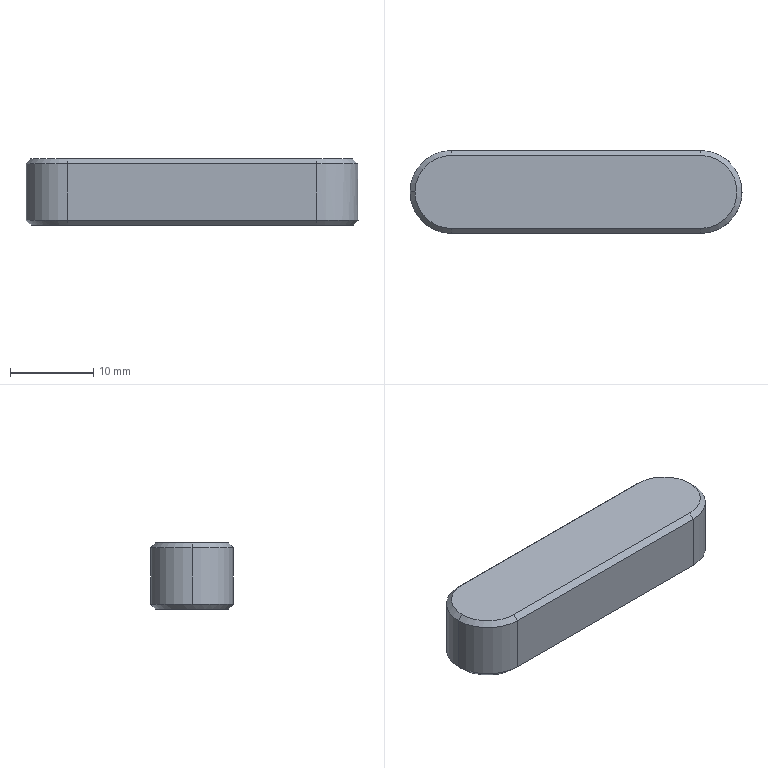Part | SolidWorks | features BaseBody 1 | 1 solid | 17 faces | box 40 x 10 x 8 mm | volume 2996 mm3 | plane 8 | cone 6 | cylinder 3 | commonest cylinder face diameters 10 x3
STEP:
#1=CARTESIAN_POINT('',(35.,-4.4,-5.));
#2=VERTEX_POINT('',#1);
#3=CARTESIAN_POINT('',(39.4,0.,-5.));
#4=VERTEX_POINT('',#3);
#5=CARTESIAN_POINT('',(35.,0.,-5.));
#6=DIRECTION('',(0.,0.,1.));
#7=DIRECTION('',(1.,0.,0.));
#8=AXIS2_PLACEMENT_3D('',#5,#6,#7);
#9=CIRCLE('',#8,4.4);
#10=EDGE_CURVE('',#2,#4,#9,.T.);
#11=ORIENTED_EDGE('',*,*,#10,.T.);
#12=CARTESIAN_POINT('',(40.,0.,-4.4));
#13=VERTEX_POINT('',#12);
#14=CARTESIAN_POINT('',(40.,0.,-4.4));
#15=DIRECTION('',(0.7071,0.,0.7071));
#16=VECTOR('',#15,1000.);
#17=LINE('',#14,#16);
#18=EDGE_CURVE('',#4,#13,#17,.T.);
#19=ORIENTED_EDGE('',*,*,#18,.T.);
#20=CARTESIAN_POINT('',(35.,-5.,-4.4));
#21=VERTEX_POINT('',#20);
#22=CARTESIAN_POINT('',(35.,0.,-4.4));
#23=DIRECTION('',(0.,0.,-1.));
#24=DIRECTION('',(0.,1.,0.));
#25=AXIS2_PLACEMENT_3D('',#22,#23,#24);
#26=CIRCLE('',#25,5.);
#27=EDGE_CURVE('',#13,#21,#26,.T.);
#28=ORIENTED_EDGE('',*,*,#27,.T.);
#29=CARTESIAN_POINT('',(35.,-4.7,-4.7));
#30=DIRECTION('',(0.,-0.7071,0.7071));
#31=VECTOR('',#30,1000.);
#32=LINE('',#29,#31);
#33=EDGE_CURVE('',#2,#21,#32,.T.);
#34=ORIENTED_EDGE('',*,*,#33,.F.);
#35=EDGE_LOOP('',(#11,#19,#28,#34));
#36=FACE_OUTER_BOUND('',#35,.T.);
#37=CARTESIAN_POINT('',(35.,0.,-4.4));
#38=DIRECTION('',(0.,0.,1.));
#39=DIRECTION('',(1.,0.,0.));
#40=AXIS2_PLACEMENT_3D('',#37,#38,#39);
#41=CONICAL_SURFACE('',#40,5.,0.7854);
#42=ADVANCED_FACE('',(#36),#41,.T.);
#43=CARTESIAN_POINT('',(5.,-5.,2.4));
#44=VERTEX_POINT('',#43);
#45=CARTESIAN_POINT('',(0.,0.,2.4));
#46=VERTEX_POINT('',#45);
#47=CARTESIAN_POINT('',(5.,0.,2.4));
#48=DIRECTION('',(0.,0.,-1.));
#49=DIRECTION('',(-1.,0.,0.));
#50=AXIS2_PLACEMENT_3D('',#47,#48,#49);
#51=CIRCLE('',#50,5.);
#52=EDGE_CURVE('',#44,#46,#51,.T.);
#53=ORIENTED_EDGE('',*,*,#52,.T.);
#54=CARTESIAN_POINT('',(0.,0.,-4.4));
#55=VERTEX_POINT('',#54);
#56=CARTESIAN_POINT('',(0.,0.,0.));
#57=DIRECTION('',(0.,0.,-1.));
#58=VECTOR('',#57,1000.);
#59=LINE('',#56,#58);
#60=EDGE_CURVE('',#46,#55,#59,.T.);
#61=ORIENTED_EDGE('',*,*,#60,.T.);
#62=CARTESIAN_POINT('',(5.,-5.,-4.4));
#63=VERTEX_POINT('',#62);
#64=CARTESIAN_POINT('',(5.,0.,-4.4));
#65=DIRECTION('',(0.,0.,-1.));
#66=DIRECTION('',(0.,-1.,0.));
#67=AXIS2_PLACEMENT_3D('',#64,#65,#66);
#68=CIRCLE('',#67,5.);
#69=EDGE_CURVE('',#63,#55,#68,.T.);
#70=ORIENTED_EDGE('',*,*,#69,.F.);
#71=CARTESIAN_POINT('',(5.,-5.,0.));
#72=DIRECTION('',(0.,0.,-1.));
#73=VECTOR('',#72,1000.);
#74=LINE('',#71,#73);
#75=EDGE_CURVE('',#44,#63,#74,.T.);
#76=ORIENTED_EDGE('',*,*,#75,.F.);
#77=EDGE_LOOP('',(#53,#61,#70,#76));
#78=FACE_OUTER_BOUND('',#77,.T.);
#79=CARTESIAN_POINT('',(5.,0.,0.));
#80=DIRECTION('',(0.,0.,-1.));
#81=DIRECTION('',(-1.,0.,0.));
#82=AXIS2_PLACEMENT_3D('',#79,#80,#81);
#83=CYLINDRICAL_SURFACE('',#82,5.);
#84=ADVANCED_FACE('',(#78),#83,.T.);
#85=CARTESIAN_POINT('',(5.,-4.4,3.));
#86=VERTEX_POINT('',#85);
#87=CARTESIAN_POINT('',(0.6,0.,3.));
#88=VERTEX_POINT('',#87);
#89=CARTESIAN_POINT('',(5.,0.,3.));
#90=DIRECTION('',(0.,0.,-1.));
#91=DIRECTION('',(-1.,0.,0.));
#92=AXIS2_PLACEMENT_3D('',#89,#90,#91);
#93=CIRCLE('',#92,4.4);
#94=EDGE_CURVE('',#86,#88,#93,.T.);
#95=ORIENTED_EDGE('',*,*,#94,.T.);
#96=CARTESIAN_POINT('',(0.,0.,2.4));
#97=DIRECTION('',(-0.7071,0.,-0.7071));
#98=VECTOR('',#97,1000.);
#99=LINE('',#96,#98);
#100=EDGE_CURVE('',#88,#46,#99,.T.);
#101=ORIENTED_EDGE('',*,*,#100,.T.);
#102=ORIENTED_EDGE('',*,*,#52,.F.);
#103=CARTESIAN_POINT('',(5.,-4.7,2.7));
#104=DIRECTION('',(0.,-0.7071,-0.7071));
#105=VECTOR('',#104,1000.);
#106=LINE('',#103,#105);
#107=EDGE_CURVE('',#86,#44,#106,.T.);
#108=ORIENTED_EDGE('',*,*,#107,.F.);
#109=EDGE_LOOP('',(#95,#101,#102,#108));
#110=FACE_OUTER_BOUND('',#109,.T.);
#111=CARTESIAN_POINT('',(5.,0.,2.4));
#112=DIRECTION('',(0.,0.,-1.));
#113=DIRECTION('',(-1.,0.,0.));
#114=AXIS2_PLACEMENT_3D('',#111,#112,#113);
#115=CONICAL_SURFACE('',#114,5.,0.7854);
#116=ADVANCED_FACE('',(#110),#115,.T.);
#117=CARTESIAN_POINT('',(5.,4.4,-5.));
#118=VERTEX_POINT('',#117);
#119=CARTESIAN_POINT('',(5.,-4.4,-5.));
#120=VERTEX_POINT('',#119);
#121=CARTESIAN_POINT('',(5.,0.,-5.));
#122=DIRECTION('',(0.,0.,1.));
#123=DIRECTION('',(1.,0.,0.));
#124=AXIS2_PLACEMENT_3D('',#121,#122,#123);
#125=CIRCLE('',#124,4.4);
#126=EDGE_CURVE('',#118,#120,#125,.T.);
#127=ORIENTED_EDGE('',*,*,#126,.F.);
#128=CARTESIAN_POINT('',(35.,4.4,-5.));
#129=VERTEX_POINT('',#128);
#130=CARTESIAN_POINT('',(20.,4.4,-5.));
#131=DIRECTION('',(-1.,0.,0.));
#132=VECTOR('',#131,1000.);
#133=LINE('',#130,#132);
#134=EDGE_CURVE('',#129,#118,#133,.T.);
#135=ORIENTED_EDGE('',*,*,#134,.F.);
#136=CARTESIAN_POINT('',(35.,0.,-5.));
#137=DIRECTION('',(0.,0.,1.));
#138=DIRECTION('',(1.,0.,0.));
#139=AXIS2_PLACEMENT_3D('',#136,#137,#138);
#140=CIRCLE('',#139,4.4);
#141=EDGE_CURVE('',#4,#129,#140,.T.);
#142=ORIENTED_EDGE('',*,*,#141,.F.);
#143=ORIENTED_EDGE('',*,*,#10,.F.);
#144=CARTESIAN_POINT('',(20.,-4.4,-5.));
#145=DIRECTION('',(1.,0.,0.));
#146=VECTOR('',#145,1000.);
#147=LINE('',#144,#146);
#148=EDGE_CURVE('',#120,#2,#147,.T.);
#149=ORIENTED_EDGE('',*,*,#148,.F.);
#150=EDGE_LOOP('',(#127,#135,#142,#143,#149));
#151=FACE_OUTER_BOUND('',#150,.T.);
#152=CARTESIAN_POINT('',(20.,0.,-5.));
#153=DIRECTION('',(0.,0.,1.));
#154=DIRECTION('',(1.,0.,0.));
#155=AXIS2_PLACEMENT_3D('',#152,#153,#154);
#156=PLANE('',#155);
#157=ADVANCED_FACE('',(#151),#156,.F.);
#158=CARTESIAN_POINT('',(5.,-4.7,-4.7));
#159=DIRECTION('',(0.,0.7071,-0.7071));
#160=VECTOR('',#159,1000.);
#161=LINE('',#158,#160);
#162=EDGE_CURVE('',#63,#120,#161,.T.);
#163=ORIENTED_EDGE('',*,*,#162,.T.);
#164=ORIENTED_EDGE('',*,*,#148,.T.);
#165=ORIENTED_EDGE('',*,*,#33,.T.);
#166=CARTESIAN_POINT('',(12.5,-5.,-4.4));
#167=DIRECTION('',(-1.,0.,0.));
#168=VECTOR('',#167,1000.);
#169=LINE('',#166,#168);
#170=EDGE_CURVE('',#21,#63,#169,.T.);
#171=ORIENTED_EDGE('',*,*,#170,.T.);
#172=EDGE_LOOP('',(#163,#164,#165,#171));
#173=FACE_OUTER_BOUND('',#172,.T.);
#174=CARTESIAN_POINT('',(12.5,-4.7,-4.7));
#175=DIRECTION('',(0.,-0.7071,-0.7071));
#176=DIRECTION('',(0.,0.7071,-0.7071));
#177=AXIS2_PLACEMENT_3D('',#174,#175,#176);
#178=PLANE('',#177);
#179=ADVANCED_FACE('',(#173),#178,.T.);
#180=ORIENTED_EDGE('',*,*,#162,.F.);
#181=ORIENTED_EDGE('',*,*,#69,.T.);
#182=CARTESIAN_POINT('',(5.,5.,-4.4));
#183=VERTEX_POINT('',#182);
#184=CARTESIAN_POINT('',(5.,0.,-4.4));
#185=DIRECTION('',(0.,0.,-1.));
#186=DIRECTION('',(0.,-1.,0.));
#187=AXIS2_PLACEMENT_3D('',#184,#185,#186);
#188=CIRCLE('',#187,5.);
#189=EDGE_CURVE('',#55,#183,#188,.T.);
#190=ORIENTED_EDGE('',*,*,#189,.T.);
#191=CARTESIAN_POINT('',(5.,499000.,498990.6));
#192=DIRECTION('',(0.,-0.7071,-0.7071));
#193=VECTOR('',#192,1000.);
#194=LINE('',#191,#193);
#195=EDGE_CURVE('',#183,#118,#194,.T.);
#196=ORIENTED_EDGE('',*,*,#195,.T.);
#197=ORIENTED_EDGE('',*,*,#126,.T.);
#198=EDGE_LOOP('',(#180,#181,#190,#196,#197));
#199=FACE_OUTER_BOUND('',#198,.T.);
#200=CARTESIAN_POINT('',(5.,0.,-4.4));
#201=DIRECTION('',(0.,0.,1.));
#202=DIRECTION('',(1.,0.,0.));
#203=AXIS2_PLACEMENT_3D('',#200,#201,#202);
#204=CONICAL_SURFACE('',#203,5.,0.7854);
#205=ADVANCED_FACE('',(#199),#204,.T.);
#206=ORIENTED_EDGE('',*,*,#195,.F.);
#207=CARTESIAN_POINT('',(35.,5.,-4.4));
#208=VERTEX_POINT('',#207);
#209=CARTESIAN_POINT('',(27.5,5.,-4.4));
#210=DIRECTION('',(1.,0.,0.));
#211=VECTOR('',#210,1000.);
#212=LINE('',#209,#211);
#213=EDGE_CURVE('',#183,#208,#212,.T.);
#214=ORIENTED_EDGE('',*,*,#213,.T.);
#215=CARTESIAN_POINT('',(35.,4.7,-4.7));
#216=DIRECTION('',(0.,-0.7071,-0.7071));
#217=VECTOR('',#216,1000.);
#218=LINE('',#215,#217);
#219=EDGE_CURVE('',#208,#129,#218,.T.);
#220=ORIENTED_EDGE('',*,*,#219,.T.);
#221=ORIENTED_EDGE('',*,*,#134,.T.);
#222=EDGE_LOOP('',(#206,#214,#220,#221));
#223=FACE_OUTER_BOUND('',#222,.T.);
#224=CARTESIAN_POINT('',(27.5,4.7,-4.7));
#225=DIRECTION('',(0.,0.7071,-0.7071));
#226=DIRECTION('',(0.,0.7071,0.7071));
#227=AXIS2_PLACEMENT_3D('',#224,#225,#226);
#228=PLANE('',#227);
#229=ADVANCED_FACE('',(#223),#228,.T.);
#230=ORIENTED_EDGE('',*,*,#18,.F.);
#231=ORIENTED_EDGE('',*,*,#141,.T.);
#232=ORIENTED_EDGE('',*,*,#219,.F.);
#233=CARTESIAN_POINT('',(35.,0.,-4.4));
#234=DIRECTION('',(0.,0.,-1.));
#235=DIRECTION('',(0.,1.,0.));
#236=AXIS2_PLACEMENT_3D('',#233,#234,#235);
#237=CIRCLE('',#236,5.);
#238=EDGE_CURVE('',#208,#13,#237,.T.);
#239=ORIENTED_EDGE('',*,*,#238,.T.);
#240=EDGE_LOOP('',(#230,#231,#232,#239));
#241=FACE_OUTER_BOUND('',#240,.T.);
#242=CARTESIAN_POINT('',(35.,0.,-4.4));
#243=DIRECTION('',(0.,0.,1.));
#244=DIRECTION('',(1.,0.,0.));
#245=AXIS2_PLACEMENT_3D('',#242,#243,#244);
#246=CONICAL_SURFACE('',#245,5.,0.7854);
#247=ADVANCED_FACE('',(#241),#246,.T.);
#248=CARTESIAN_POINT('',(35.,-5.,2.4));
#249=VERTEX_POINT('',#248);
#250=CARTESIAN_POINT('',(5.,-5.,2.4));
#251=DIRECTION('',(-1.,0.,0.));
#252=VECTOR('',#251,1000.);
#253=LINE('',#250,#252);
#254=EDGE_CURVE('',#249,#44,#253,.T.);
#255=ORIENTED_EDGE('',*,*,#254,.T.);
#256=ORIENTED_EDGE('',*,*,#75,.T.);
#257=ORIENTED_EDGE('',*,*,#170,.F.);
#258=CARTESIAN_POINT('',(35.,-5.,0.));
#259=DIRECTION('',(0.,0.,1.));
#260=VECTOR('',#259,1000.);
#261=LINE('',#258,#260);
#262=EDGE_CURVE('',#21,#249,#261,.T.);
#263=ORIENTED_EDGE('',*,*,#262,.T.);
#264=EDGE_LOOP('',(#255,#256,#257,#263));
#265=FACE_OUTER_BOUND('',#264,.T.);
#266=CARTESIAN_POINT('',(5.,-5.,0.));
#267=DIRECTION('',(0.,-1.,0.));
#268=DIRECTION('',(1.,0.,0.));
#269=AXIS2_PLACEMENT_3D('',#266,#267,#268);
#270=PLANE('',#269);
#271=ADVANCED_FACE('',(#265),#270,.T.);
#272=ORIENTED_EDGE('',*,*,#60,.F.);
#273=CARTESIAN_POINT('',(5.,5.,2.4));
#274=VERTEX_POINT('',#273);
#275=CARTESIAN_POINT('',(5.,0.,2.4));
#276=DIRECTION('',(0.,0.,-1.));
#277=DIRECTION('',(-1.,0.,0.));
#278=AXIS2_PLACEMENT_3D('',#275,#276,#277);
#279=CIRCLE('',#278,5.);
#280=EDGE_CURVE('',#46,#274,#279,.T.);
#281=ORIENTED_EDGE('',*,*,#280,.T.);
#282=CARTESIAN_POINT('',(5.,5.,0.));
#283=DIRECTION('',(0.,0.,-1.));
#284=VECTOR('',#283,1000.);
#285=LINE('',#282,#284);
#286=EDGE_CURVE('',#274,#183,#285,.T.);
#287=ORIENTED_EDGE('',*,*,#286,.T.);
#288=ORIENTED_EDGE('',*,*,#189,.F.);
#289=EDGE_LOOP('',(#272,#281,#287,#288));
#290=FACE_OUTER_BOUND('',#289,.T.);
#291=CARTESIAN_POINT('',(5.,0.,0.));
#292=DIRECTION('',(0.,0.,-1.));
#293=DIRECTION('',(-1.,0.,0.));
#294=AXIS2_PLACEMENT_3D('',#291,#292,#293);
#295=CYLINDRICAL_SURFACE('',#294,5.);
#296=ADVANCED_FACE('',(#290),#295,.T.);
#297=CARTESIAN_POINT('',(35.,5.,2.4));
#298=VERTEX_POINT('',#297);
#299=CARTESIAN_POINT('',(35.,5.,2.4));
#300=DIRECTION('',(1.,0.,0.));
#301=VECTOR('',#300,1000.);
#302=LINE('',#299,#301);
#303=EDGE_CURVE('',#274,#298,#302,.T.);
#304=ORIENTED_EDGE('',*,*,#303,.T.);
#305=CARTESIAN_POINT('',(35.,5.,0.));
#306=DIRECTION('',(0.,0.,-1.));
#307=VECTOR('',#306,1000.);
#308=LINE('',#305,#307);
#309=EDGE_CURVE('',#298,#208,#308,.T.);
#310=ORIENTED_EDGE('',*,*,#309,.T.);
#311=ORIENTED_EDGE('',*,*,#213,.F.);
#312=ORIENTED_EDGE('',*,*,#286,.F.);
#313=EDGE_LOOP('',(#304,#310,#311,#312));
#314=FACE_OUTER_BOUND('',#313,.T.);
#315=CARTESIAN_POINT('',(35.,5.,0.));
#316=DIRECTION('',(0.,1.,0.));
#317=DIRECTION('',(0.,0.,1.));
#318=AXIS2_PLACEMENT_3D('',#315,#316,#317);
#319=PLANE('',#318);
#320=ADVANCED_FACE('',(#314),#319,.T.);
#321=CARTESIAN_POINT('',(35.,0.,2.4));
#322=DIRECTION('',(0.,0.,-1.));
#323=DIRECTION('',(-1.,0.,0.));
#324=AXIS2_PLACEMENT_3D('',#321,#322,#323);
#325=CIRCLE('',#324,5.);
#326=EDGE_CURVE('',#298,#249,#325,.T.);
#327=ORIENTED_EDGE('',*,*,#326,.T.);
#328=ORIENTED_EDGE('',*,*,#262,.F.);
#329=ORIENTED_EDGE('',*,*,#27,.F.);
#330=ORIENTED_EDGE('',*,*,#238,.F.);
#331=ORIENTED_EDGE('',*,*,#309,.F.);
#332=EDGE_LOOP('',(#327,#328,#329,#330,#331));
#333=FACE_OUTER_BOUND('',#332,.T.);
#334=CARTESIAN_POINT('',(35.,0.,0.));
#335=DIRECTION('',(0.,0.,-1.));
#336=DIRECTION('',(-1.,0.,0.));
#337=AXIS2_PLACEMENT_3D('',#334,#335,#336);
#338=CYLINDRICAL_SURFACE('',#337,5.);
#339=ADVANCED_FACE('',(#333),#338,.T.);
#340=ORIENTED_EDGE('',*,*,#107,.T.);
#341=ORIENTED_EDGE('',*,*,#254,.F.);
#342=CARTESIAN_POINT('',(35.,-4.4,3.));
#343=VERTEX_POINT('',#342);
#344=CARTESIAN_POINT('',(35.,-4.7,2.7));
#345=DIRECTION('',(0.,0.7071,0.7071));
#346=VECTOR('',#345,1000.);
#347=LINE('',#344,#346);
#348=EDGE_CURVE('',#249,#343,#347,.T.);
#349=ORIENTED_EDGE('',*,*,#348,.T.);
#350=CARTESIAN_POINT('',(12.5,-4.4,3.));
#351=DIRECTION('',(-1.,0.,0.));
#352=VECTOR('',#351,1000.);
#353=LINE('',#350,#352);
#354=EDGE_CURVE('',#343,#86,#353,.T.);
#355=ORIENTED_EDGE('',*,*,#354,.T.);
#356=EDGE_LOOP('',(#340,#341,#349,#355));
#357=FACE_OUTER_BOUND('',#356,.T.);
#358=CARTESIAN_POINT('',(12.5,-4.7,2.7));
#359=DIRECTION('',(0.,-0.7071,0.7071));
#360=DIRECTION('',(0.,-0.7071,-0.7071));
#361=AXIS2_PLACEMENT_3D('',#358,#359,#360);
#362=PLANE('',#361);
#363=ADVANCED_FACE('',(#357),#362,.T.);
#364=ORIENTED_EDGE('',*,*,#100,.F.);
#365=CARTESIAN_POINT('',(5.,4.4,3.));
#366=VERTEX_POINT('',#365);
#367=CARTESIAN_POINT('',(5.,0.,3.));
#368=DIRECTION('',(0.,0.,-1.));
#369=DIRECTION('',(-1.,0.,0.));
#370=AXIS2_PLACEMENT_3D('',#367,#368,#369);
#371=CIRCLE('',#370,4.4);
#372=EDGE_CURVE('',#88,#366,#371,.T.);
#373=ORIENTED_EDGE('',*,*,#372,.T.);
#374=CARTESIAN_POINT('',(5.,499000.,-498992.6));
#375=DIRECTION('',(0.,0.7071,-0.7071));
#376=VECTOR('',#375,1000.);
#377=LINE('',#374,#376);
#378=EDGE_CURVE('',#366,#274,#377,.T.);
#379=ORIENTED_EDGE('',*,*,#378,.T.);
#380=ORIENTED_EDGE('',*,*,#280,.F.);
#381=EDGE_LOOP('',(#364,#373,#379,#380));
#382=FACE_OUTER_BOUND('',#381,.T.);
#383=CARTESIAN_POINT('',(5.,0.,2.4));
#384=DIRECTION('',(0.,0.,-1.));
#385=DIRECTION('',(-1.,0.,0.));
#386=AXIS2_PLACEMENT_3D('',#383,#384,#385);
#387=CONICAL_SURFACE('',#386,5.,0.7854);
#388=ADVANCED_FACE('',(#382),#387,.T.);
#389=ORIENTED_EDGE('',*,*,#378,.F.);
#390=CARTESIAN_POINT('',(35.,4.4,3.));
#391=VERTEX_POINT('',#390);
#392=CARTESIAN_POINT('',(27.5,4.4,3.));
#393=DIRECTION('',(1.,0.,0.));
#394=VECTOR('',#393,1000.);
#395=LINE('',#392,#394);
#396=EDGE_CURVE('',#366,#391,#395,.T.);
#397=ORIENTED_EDGE('',*,*,#396,.T.);
#398=CARTESIAN_POINT('',(35.,4.7,2.7));
#399=DIRECTION('',(0.,0.7071,-0.7071));
#400=VECTOR('',#399,1000.);
#401=LINE('',#398,#400);
#402=EDGE_CURVE('',#391,#298,#401,.T.);
#403=ORIENTED_EDGE('',*,*,#402,.T.);
#404=ORIENTED_EDGE('',*,*,#303,.F.);
#405=EDGE_LOOP('',(#389,#397,#403,#404));
#406=FACE_OUTER_BOUND('',#405,.T.);
#407=CARTESIAN_POINT('',(27.5,4.7,2.7));
#408=DIRECTION('',(0.,0.7071,0.7071));
#409=DIRECTION('',(0.,-0.7071,0.7071));
#410=AXIS2_PLACEMENT_3D('',#407,#408,#409);
#411=PLANE('',#410);
#412=ADVANCED_FACE('',(#406),#411,.T.);
#413=ORIENTED_EDGE('',*,*,#402,.F.);
#414=CARTESIAN_POINT('',(35.,0.,3.));
#415=DIRECTION('',(0.,0.,-1.));
#416=DIRECTION('',(-1.,0.,0.));
#417=AXIS2_PLACEMENT_3D('',#414,#415,#416);
#418=CIRCLE('',#417,4.4);
#419=EDGE_CURVE('',#391,#343,#418,.T.);
#420=ORIENTED_EDGE('',*,*,#419,.T.);
#421=ORIENTED_EDGE('',*,*,#348,.F.);
#422=ORIENTED_EDGE('',*,*,#326,.F.);
#423=EDGE_LOOP('',(#413,#420,#421,#422));
#424=FACE_OUTER_BOUND('',#423,.T.);
#425=CARTESIAN_POINT('',(35.,0.,2.4));
#426=DIRECTION('',(0.,0.,-1.));
#427=DIRECTION('',(-1.,0.,0.));
#428=AXIS2_PLACEMENT_3D('',#425,#426,#427);
#429=CONICAL_SURFACE('',#428,5.,0.7854);
#430=ADVANCED_FACE('',(#424),#429,.T.);
#431=ORIENTED_EDGE('',*,*,#419,.F.);
#432=ORIENTED_EDGE('',*,*,#396,.F.);
#433=ORIENTED_EDGE('',*,*,#372,.F.);
#434=ORIENTED_EDGE('',*,*,#94,.F.);
#435=ORIENTED_EDGE('',*,*,#354,.F.);
#436=EDGE_LOOP('',(#431,#432,#433,#434,#435));
#437=FACE_OUTER_BOUND('',#436,.T.);
#438=CARTESIAN_POINT('',(20.,0.,3.));
#439=DIRECTION('',(0.,0.,1.));
#440=DIRECTION('',(1.,0.,0.));
#441=AXIS2_PLACEMENT_3D('',#438,#439,#440);
#442=PLANE('',#441);
#443=ADVANCED_FACE('',(#437),#442,.T.);
#444=CLOSED_SHELL('',(#42,#84,#116,#157,#179,#205,#229,#247,#271,#296,#320,#339,#363,#388,#412,#430,#443));
#445=MANIFOLD_SOLID_BREP('',#444);
#446=CARTESIAN_POINT('',(0.,0.,0.));
#447=DIRECTION('',(0.,0.,1.));
#448=DIRECTION('',(1.,0.,0.));
#449=AXIS2_PLACEMENT_3D('',#446,#447,#448);
#450=(LENGTH_UNIT()NAMED_UNIT(*)SI_UNIT(.MILLI.,.METRE.));
#451=UNCERTAINTY_MEASURE_WITH_UNIT(LENGTH_MEASURE(0.00001),#450,'','');
#452=(NAMED_UNIT(*)PLANE_ANGLE_UNIT()SI_UNIT($,.RADIAN.));
#453=(NAMED_UNIT(*)SI_UNIT($,.STERADIAN.)SOLID_ANGLE_UNIT());
#454=(GEOMETRIC_REPRESENTATION_CONTEXT(3)GLOBAL_UNCERTAINTY_ASSIGNED_CONTEXT((#451))GLOBAL_UNIT_ASSIGNED_CONTEXT((#450,#452,#453))REPRESENTATION_CONTEXT('',''));
#455=ADVANCED_BREP_SHAPE_REPRESENTATION('',(#445,#449),#454);